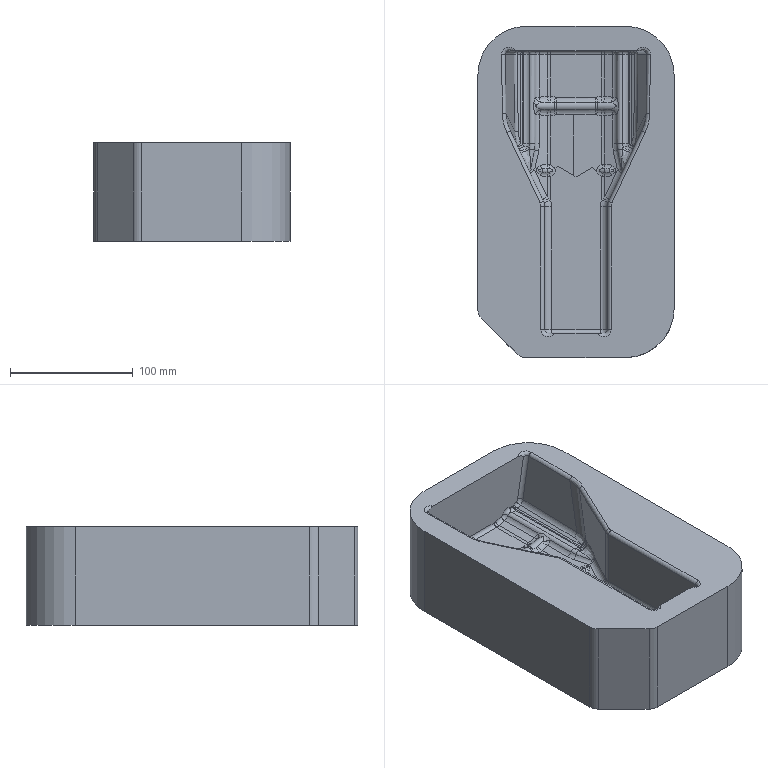Part | 1 solid | 183 faces | box 160 x 270 x 80 mm | volume 2415379 mm3 | cylinder 62 | spline 62 | plane 27 | torus 24 | sphere 8 | commonest cylinder face diameters 6 x22 12 x16 20 x10 7 x4 8 x3 80 x3